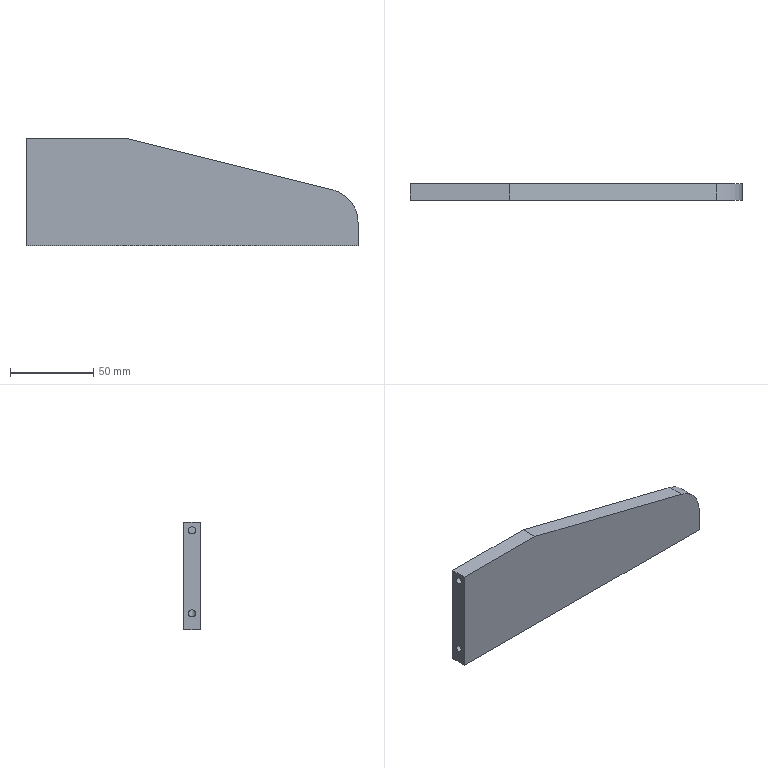Part | STEP file | PN_0004 | 1 solid | 23 faces | box 200 x 10 x 65 mm | volume 103240 mm3 | cylinder 12 | plane 11 | commonest cylinder face diameters 4.3 x11 40 x1